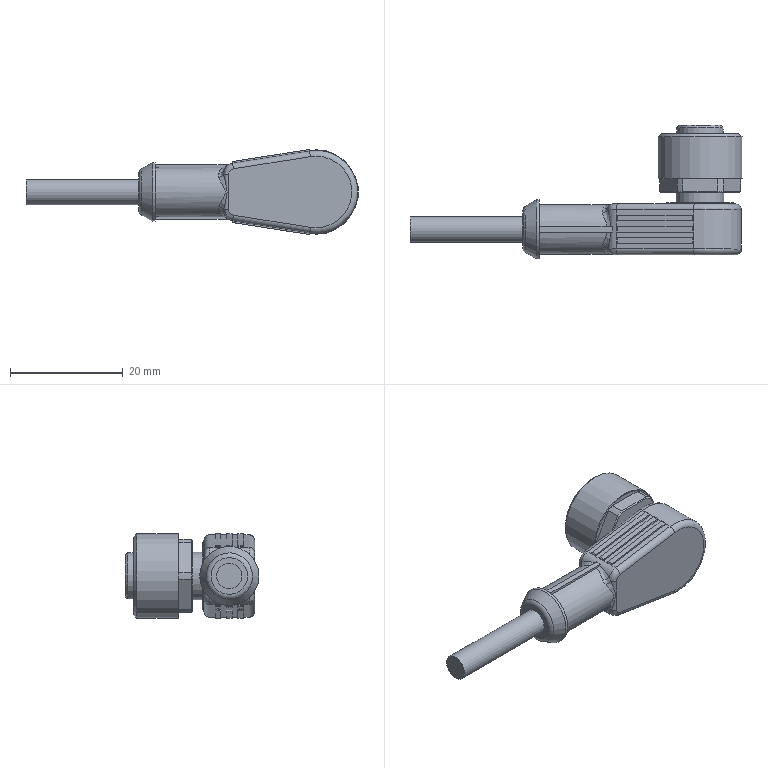Part | NX | features BREP 1 | 1 solid | 153 faces | box 59 x 23.75 x 15.058 mm | volume 5436 mm3 | plane 79 | cylinder 45 | spline 14 | cone 11 | torus 4 | commonest cylinder face diameters 0.4 x12 2 x6 14.4 x6 1.2 x5 4.8 x4 4 x2